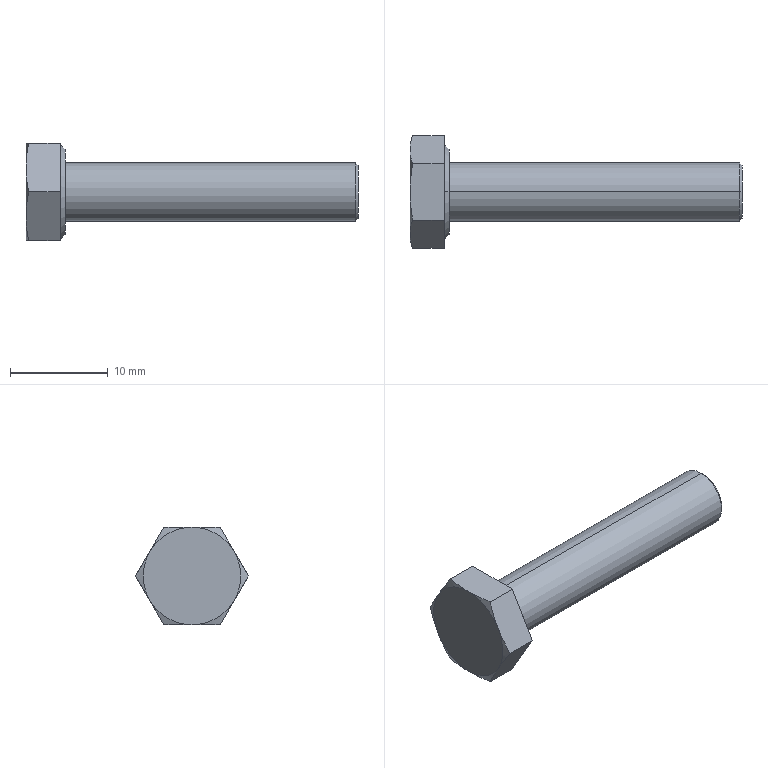Part | SolidWorks | features RevCut 3, Boss 1, Chamfer 1, Extrusion 1, Fillet 1, LPattern 1 | 1 solid | 22 faces | box 34 x 11.547 x 10 mm | volume 1183 mm3 | cone 10 | plane 10 | cylinder 2 | commonest cylinder face diameters 6 x2
STEP:
#1=CARTESIAN_POINT('',(34.,0.,-2.7));
#2=VERTEX_POINT('',#1);
#3=CARTESIAN_POINT('',(34.,0.,2.7));
#4=VERTEX_POINT('',#3);
#5=CARTESIAN_POINT('',(34.,0.,0.));
#6=DIRECTION('',(1.,0.,0.));
#7=DIRECTION('',(0.,0.,-1.));
#8=AXIS2_PLACEMENT_3D('',#5,#6,#7);
#9=CIRCLE('',#8,2.7);
#10=EDGE_CURVE('',#2,#4,#9,.T.);
#11=ORIENTED_EDGE('',*,*,#10,.F.);
#12=CARTESIAN_POINT('',(33.7,0.,-3.));
#13=VERTEX_POINT('',#12);
#14=CARTESIAN_POINT('',(34.,0.,-2.7));
#15=DIRECTION('',(-0.7071,0.,-0.7071));
#16=VECTOR('',#15,1000.);
#17=LINE('',#14,#16);
#18=EDGE_CURVE('',#2,#13,#17,.T.);
#19=ORIENTED_EDGE('',*,*,#18,.T.);
#20=CARTESIAN_POINT('',(33.7,0.,3.));
#21=VERTEX_POINT('',#20);
#22=CARTESIAN_POINT('',(33.7,0.,0.));
#23=DIRECTION('',(-1.,0.,0.));
#24=DIRECTION('',(0.,0.,-1.));
#25=AXIS2_PLACEMENT_3D('',#22,#23,#24);
#26=CIRCLE('',#25,3.);
#27=EDGE_CURVE('',#21,#13,#26,.T.);
#28=ORIENTED_EDGE('',*,*,#27,.F.);
#29=CARTESIAN_POINT('',(34.,0.,2.7));
#30=DIRECTION('',(-0.7071,0.,0.7071));
#31=VECTOR('',#30,1000.);
#32=LINE('',#29,#31);
#33=EDGE_CURVE('',#4,#21,#32,.T.);
#34=ORIENTED_EDGE('',*,*,#33,.F.);
#35=EDGE_LOOP('',(#11,#19,#28,#34));
#36=FACE_OUTER_BOUND('',#35,.T.);
#37=CARTESIAN_POINT('',(34.,0.,0.));
#38=DIRECTION('',(-1.,0.,0.));
#39=DIRECTION('',(0.,0.,1.));
#40=AXIS2_PLACEMENT_3D('',#37,#38,#39);
#41=CONICAL_SURFACE('',#40,2.7,0.7854);
#42=ADVANCED_FACE('',(#36),#41,.T.);
#43=ORIENTED_EDGE('',*,*,#27,.T.);
#44=CARTESIAN_POINT('',(4.,0.,-3.));
#45=VERTEX_POINT('',#44);
#46=CARTESIAN_POINT('',(34.,0.,-3.));
#47=DIRECTION('',(-1.,0.,0.));
#48=VECTOR('',#47,1000.);
#49=LINE('',#46,#48);
#50=EDGE_CURVE('',#13,#45,#49,.T.);
#51=ORIENTED_EDGE('',*,*,#50,.T.);
#52=CARTESIAN_POINT('',(4.,0.,3.));
#53=VERTEX_POINT('',#52);
#54=CARTESIAN_POINT('',(4.,0.,0.));
#55=DIRECTION('',(1.,0.,0.));
#56=DIRECTION('',(0.,0.,-1.));
#57=AXIS2_PLACEMENT_3D('',#54,#55,#56);
#58=CIRCLE('',#57,3.);
#59=EDGE_CURVE('',#45,#53,#58,.T.);
#60=ORIENTED_EDGE('',*,*,#59,.T.);
#61=CARTESIAN_POINT('',(34.,0.,3.));
#62=DIRECTION('',(-1.,0.,0.));
#63=VECTOR('',#62,1000.);
#64=LINE('',#61,#63);
#65=EDGE_CURVE('',#21,#53,#64,.T.);
#66=ORIENTED_EDGE('',*,*,#65,.F.);
#67=EDGE_LOOP('',(#43,#51,#60,#66));
#68=FACE_OUTER_BOUND('',#67,.T.);
#69=CARTESIAN_POINT('',(34.,0.,0.));
#70=DIRECTION('',(-1.,0.,0.));
#71=DIRECTION('',(0.,0.,1.));
#72=AXIS2_PLACEMENT_3D('',#69,#70,#71);
#73=CYLINDRICAL_SURFACE('',#72,3.);
#74=ADVANCED_FACE('',(#68),#73,.T.);
#75=CARTESIAN_POINT('',(4.,0.,4.37));
#76=VERTEX_POINT('',#75);
#77=CARTESIAN_POINT('',(4.,0.,-4.37));
#78=VERTEX_POINT('',#77);
#79=CARTESIAN_POINT('',(4.,0.,0.));
#80=DIRECTION('',(-1.,0.,0.));
#81=DIRECTION('',(0.,0.,1.));
#82=AXIS2_PLACEMENT_3D('',#79,#80,#81);
#83=CIRCLE('',#82,4.37);
#84=EDGE_CURVE('',#76,#78,#83,.T.);
#85=ORIENTED_EDGE('',*,*,#84,.T.);
#86=CARTESIAN_POINT('',(3.5,0.,-4.87));
#87=VERTEX_POINT('',#86);
#88=CARTESIAN_POINT('',(3.5,0.,-4.87));
#89=DIRECTION('',(-0.7071,0.,-0.7071));
#90=VECTOR('',#89,1000.);
#91=LINE('',#88,#90);
#92=EDGE_CURVE('',#78,#87,#91,.T.);
#93=ORIENTED_EDGE('',*,*,#92,.T.);
#94=CARTESIAN_POINT('',(3.5,0.,4.87));
#95=VERTEX_POINT('',#94);
#96=CARTESIAN_POINT('',(3.5,0.,0.));
#97=DIRECTION('',(-1.,0.,0.));
#98=DIRECTION('',(0.,0.,1.));
#99=AXIS2_PLACEMENT_3D('',#96,#97,#98);
#100=CIRCLE('',#99,4.87);
#101=EDGE_CURVE('',#95,#87,#100,.T.);
#102=ORIENTED_EDGE('',*,*,#101,.F.);
#103=CARTESIAN_POINT('',(3.5,0.,4.87));
#104=DIRECTION('',(-0.7071,0.,0.7071));
#105=VECTOR('',#104,1000.);
#106=LINE('',#103,#105);
#107=EDGE_CURVE('',#76,#95,#106,.T.);
#108=ORIENTED_EDGE('',*,*,#107,.F.);
#109=EDGE_LOOP('',(#85,#93,#102,#108));
#110=FACE_OUTER_BOUND('',#109,.T.);
#111=CARTESIAN_POINT('',(3.5,0.,0.));
#112=DIRECTION('',(-1.,0.,0.));
#113=DIRECTION('',(0.,0.,1.));
#114=AXIS2_PLACEMENT_3D('',#111,#112,#113);
#115=CONICAL_SURFACE('',#114,4.87,0.7854);
#116=ADVANCED_FACE('',(#110),#115,.T.);
#117=ORIENTED_EDGE('',*,*,#84,.F.);
#118=CARTESIAN_POINT('',(4.,0.,0.));
#119=DIRECTION('',(-1.,0.,0.));
#120=DIRECTION('',(0.,0.,1.));
#121=AXIS2_PLACEMENT_3D('',#118,#119,#120);
#122=CIRCLE('',#121,4.37);
#123=EDGE_CURVE('',#78,#76,#122,.T.);
#124=ORIENTED_EDGE('',*,*,#123,.F.);
#125=EDGE_LOOP('',(#117,#124));
#126=FACE_OUTER_BOUND('',#125,.T.);
#127=CARTESIAN_POINT('',(4.,0.,0.));
#128=DIRECTION('',(1.,0.,0.));
#129=DIRECTION('',(0.,0.,-1.));
#130=AXIS2_PLACEMENT_3D('',#127,#128,#129);
#131=CIRCLE('',#130,3.);
#132=EDGE_CURVE('',#53,#45,#131,.T.);
#133=ORIENTED_EDGE('',*,*,#132,.F.);
#134=ORIENTED_EDGE('',*,*,#59,.F.);
#135=EDGE_LOOP('',(#133,#134));
#136=FACE_BOUND('',#135,.T.);
#137=CARTESIAN_POINT('',(4.,-8.66,-5.));
#138=DIRECTION('',(1.,0.,0.));
#139=DIRECTION('',(0.,0.,-1.));
#140=AXIS2_PLACEMENT_3D('',#137,#138,#139);
#141=PLANE('',#140);
#142=ADVANCED_FACE('',(#126,#136),#141,.T.);
#143=CARTESIAN_POINT('',(0.2815,-5.774,0.));
#144=VERTEX_POINT('',#143);
#145=CARTESIAN_POINT('',(0.,-4.33,2.5));
#146=VERTEX_POINT('',#145);
#147=CARTESIAN_POINT('',(0.2815,-5.774,0.));
#148=CARTESIAN_POINT('',(0.1064,-5.292,0.8333));
#149=CARTESIAN_POINT('',(0.,-4.811,1.667));
#150=CARTESIAN_POINT('',(0.,-4.33,2.5));
#151=B_SPLINE_CURVE_WITH_KNOTS('',3,(#147,#148,#149,#150),.UNSPECIFIED.,.F.,.F.,(4,4),(0.000000231,0.002887),.UNSPECIFIED.);
#152=EDGE_CURVE('',#144,#146,#151,.T.);
#153=ORIENTED_EDGE('',*,*,#152,.F.);
#154=CARTESIAN_POINT('',(3.5,-5.774,0.));
#155=VERTEX_POINT('',#154);
#156=CARTESIAN_POINT('',(4.,-5.774,0.));
#157=DIRECTION('',(-1.,0.,0.));
#158=VECTOR('',#157,1000.);
#159=LINE('',#156,#158);
#160=EDGE_CURVE('',#155,#144,#159,.T.);
#161=ORIENTED_EDGE('',*,*,#160,.F.);
#162=CARTESIAN_POINT('',(3.5,-2.887,5.));
#163=VERTEX_POINT('',#162);
#164=CARTESIAN_POINT('',(3.5,-2.887,5.));
#165=DIRECTION('',(0.,-0.5,-0.866));
#166=VECTOR('',#165,1000.);
#167=LINE('',#164,#166);
#168=EDGE_CURVE('',#163,#155,#167,.T.);
#169=ORIENTED_EDGE('',*,*,#168,.F.);
#170=CARTESIAN_POINT('',(0.2815,-2.887,5.));
#171=VERTEX_POINT('',#170);
#172=CARTESIAN_POINT('',(4.,-2.887,5.));
#173=DIRECTION('',(-1.,0.,0.));
#174=VECTOR('',#173,1000.);
#175=LINE('',#172,#174);
#176=EDGE_CURVE('',#163,#171,#175,.T.);
#177=ORIENTED_EDGE('',*,*,#176,.T.);
#178=CARTESIAN_POINT('',(0.,-4.33,2.5));
#179=CARTESIAN_POINT('',(0.,-3.849,3.333));
#180=CARTESIAN_POINT('',(0.1064,-3.368,4.167));
#181=CARTESIAN_POINT('',(0.2815,-2.887,5.));
#182=B_SPLINE_CURVE_WITH_KNOTS('',3,(#178,#179,#180,#181),.UNSPECIFIED.,.F.,.F.,(4,4),(0.002887,0.005774),.UNSPECIFIED.);
#183=EDGE_CURVE('',#146,#171,#182,.T.);
#184=ORIENTED_EDGE('',*,*,#183,.F.);
#185=EDGE_LOOP('',(#153,#161,#169,#177,#184));
#186=FACE_OUTER_BOUND('',#185,.T.);
#187=CARTESIAN_POINT('',(4.,-2.887,5.));
#188=DIRECTION('',(0.,0.866,-0.5));
#189=DIRECTION('',(0.,0.5,0.866));
#190=AXIS2_PLACEMENT_3D('',#187,#188,#189);
#191=PLANE('',#190);
#192=ADVANCED_FACE('',(#186),#191,.F.);
#193=CARTESIAN_POINT('',(0.2815,-2.887,-5.));
#194=VERTEX_POINT('',#193);
#195=CARTESIAN_POINT('',(0.,-4.33,-2.5));
#196=VERTEX_POINT('',#195);
#197=CARTESIAN_POINT('',(0.2815,-2.887,-5.));
#198=CARTESIAN_POINT('',(0.1064,-3.368,-4.167));
#199=CARTESIAN_POINT('',(0.,-3.849,-3.333));
#200=CARTESIAN_POINT('',(0.,-4.33,-2.5));
#201=B_SPLINE_CURVE_WITH_KNOTS('',3,(#197,#198,#199,#200),.UNSPECIFIED.,.F.,.F.,(4,4),(0.000000231,0.002887),.UNSPECIFIED.);
#202=EDGE_CURVE('',#194,#196,#201,.T.);
#203=ORIENTED_EDGE('',*,*,#202,.F.);
#204=CARTESIAN_POINT('',(3.5,-2.887,-5.));
#205=VERTEX_POINT('',#204);
#206=CARTESIAN_POINT('',(4.,-2.887,-5.));
#207=DIRECTION('',(-1.,0.,0.));
#208=VECTOR('',#207,1000.);
#209=LINE('',#206,#208);
#210=EDGE_CURVE('',#205,#194,#209,.T.);
#211=ORIENTED_EDGE('',*,*,#210,.F.);
#212=CARTESIAN_POINT('',(3.5,-5.774,0.));
#213=DIRECTION('',(0.,0.5,-0.866));
#214=VECTOR('',#213,1000.);
#215=LINE('',#212,#214);
#216=EDGE_CURVE('',#155,#205,#215,.T.);
#217=ORIENTED_EDGE('',*,*,#216,.F.);
#218=ORIENTED_EDGE('',*,*,#160,.T.);
#219=CARTESIAN_POINT('',(0.,-4.33,-2.5));
#220=CARTESIAN_POINT('',(0.,-4.811,-1.667));
#221=CARTESIAN_POINT('',(0.1064,-5.292,-0.8333));
#222=CARTESIAN_POINT('',(0.2815,-5.774,0.));
#223=B_SPLINE_CURVE_WITH_KNOTS('',3,(#219,#220,#221,#222),.UNSPECIFIED.,.F.,.F.,(4,4),(0.002887,0.005774),.UNSPECIFIED.);
#224=EDGE_CURVE('',#196,#144,#223,.T.);
#225=ORIENTED_EDGE('',*,*,#224,.F.);
#226=EDGE_LOOP('',(#203,#211,#217,#218,#225));
#227=FACE_OUTER_BOUND('',#226,.T.);
#228=CARTESIAN_POINT('',(4.,-5.774,0.));
#229=DIRECTION('',(0.,0.866,0.5));
#230=DIRECTION('',(0.,-0.5,0.866));
#231=AXIS2_PLACEMENT_3D('',#228,#229,#230);
#232=PLANE('',#231);
#233=ADVANCED_FACE('',(#227),#232,.F.);
#234=CARTESIAN_POINT('',(0.2815,2.887,-5.));
#235=VERTEX_POINT('',#234);
#236=CARTESIAN_POINT('',(0.,0.,-5.));
#237=VERTEX_POINT('',#236);
#238=CARTESIAN_POINT('',(0.2815,2.887,-5.));
#239=CARTESIAN_POINT('',(0.1069,1.927,-5.));
#240=CARTESIAN_POINT('',(0.,0.9642,-5.));
#241=CARTESIAN_POINT('',(0.,0.,-5.));
#242=B_SPLINE_CURVE_WITH_KNOTS('',3,(#238,#239,#240,#241),.UNSPECIFIED.,.F.,.F.,(4,4),(0.01041,0.01332),.UNSPECIFIED.);
#243=EDGE_CURVE('',#235,#237,#242,.T.);
#244=ORIENTED_EDGE('',*,*,#243,.F.);
#245=CARTESIAN_POINT('',(3.5,2.887,-5.));
#246=VERTEX_POINT('',#245);
#247=CARTESIAN_POINT('',(4.,2.887,-5.));
#248=DIRECTION('',(-1.,0.,0.));
#249=VECTOR('',#248,1000.);
#250=LINE('',#247,#249);
#251=EDGE_CURVE('',#246,#235,#250,.T.);
#252=ORIENTED_EDGE('',*,*,#251,.F.);
#253=CARTESIAN_POINT('',(3.5,-2.887,-5.));
#254=DIRECTION('',(0.,1.,0.));
#255=VECTOR('',#254,1000.);
#256=LINE('',#253,#255);
#257=EDGE_CURVE('',#205,#246,#256,.T.);
#258=ORIENTED_EDGE('',*,*,#257,.F.);
#259=ORIENTED_EDGE('',*,*,#210,.T.);
#260=CARTESIAN_POINT('',(0.,0.,-5.));
#261=CARTESIAN_POINT('',(0.,-0.4807,-5.));
#262=CARTESIAN_POINT('',(0.02571,-0.962,-5.));
#263=CARTESIAN_POINT('',(0.123,-1.926,-5.));
#264=CARTESIAN_POINT('',(0.1945,-2.409,-5.));
#265=CARTESIAN_POINT('',(0.2815,-2.887,-5.));
#266=B_SPLINE_CURVE_WITH_KNOTS('',3,(#260,#261,#262,#263,#264,#265),.UNSPECIFIED.,.F.,.F.,(4,2,4),(0.01332,0.01477,0.01622),.UNSPECIFIED.);
#267=EDGE_CURVE('',#237,#194,#266,.T.);
#268=ORIENTED_EDGE('',*,*,#267,.F.);
#269=EDGE_LOOP('',(#244,#252,#258,#259,#268));
#270=FACE_OUTER_BOUND('',#269,.T.);
#271=CARTESIAN_POINT('',(4.,-2.887,-5.));
#272=DIRECTION('',(0.,0.,1.));
#273=DIRECTION('',(1.,0.,0.));
#274=AXIS2_PLACEMENT_3D('',#271,#272,#273);
#275=PLANE('',#274);
#276=ADVANCED_FACE('',(#270),#275,.F.);
#277=CARTESIAN_POINT('',(0.2815,5.774,0.));
#278=VERTEX_POINT('',#277);
#279=CARTESIAN_POINT('',(0.,4.33,-2.5));
#280=VERTEX_POINT('',#279);
#281=CARTESIAN_POINT('',(0.2815,5.774,0.));
#282=CARTESIAN_POINT('',(0.1064,5.292,-0.8333));
#283=CARTESIAN_POINT('',(0.,4.811,-1.667));
#284=CARTESIAN_POINT('',(0.,4.33,-2.5));
#285=B_SPLINE_CURVE_WITH_KNOTS('',3,(#281,#282,#283,#284),.UNSPECIFIED.,.F.,.F.,(4,4),(0.000000231,0.002887),.UNSPECIFIED.);
#286=EDGE_CURVE('',#278,#280,#285,.T.);
#287=ORIENTED_EDGE('',*,*,#286,.F.);
#288=CARTESIAN_POINT('',(3.5,5.774,0.));
#289=VERTEX_POINT('',#288);
#290=CARTESIAN_POINT('',(4.,5.774,0.));
#291=DIRECTION('',(-1.,0.,0.));
#292=VECTOR('',#291,1000.);
#293=LINE('',#290,#292);
#294=EDGE_CURVE('',#289,#278,#293,.T.);
#295=ORIENTED_EDGE('',*,*,#294,.F.);
#296=CARTESIAN_POINT('',(3.5,2.887,-5.));
#297=DIRECTION('',(0.,0.5,0.866));
#298=VECTOR('',#297,1000.);
#299=LINE('',#296,#298);
#300=EDGE_CURVE('',#246,#289,#299,.T.);
#301=ORIENTED_EDGE('',*,*,#300,.F.);
#302=ORIENTED_EDGE('',*,*,#251,.T.);
#303=CARTESIAN_POINT('',(0.,4.33,-2.5));
#304=CARTESIAN_POINT('',(0.,3.849,-3.333));
#305=CARTESIAN_POINT('',(0.1064,3.368,-4.167));
#306=CARTESIAN_POINT('',(0.2815,2.887,-5.));
#307=B_SPLINE_CURVE_WITH_KNOTS('',3,(#303,#304,#305,#306),.UNSPECIFIED.,.F.,.F.,(4,4),(0.002887,0.005774),.UNSPECIFIED.);
#308=EDGE_CURVE('',#280,#235,#307,.T.);
#309=ORIENTED_EDGE('',*,*,#308,.F.);
#310=EDGE_LOOP('',(#287,#295,#301,#302,#309));
#311=FACE_OUTER_BOUND('',#310,.T.);
#312=CARTESIAN_POINT('',(4.,2.887,-5.));
#313=DIRECTION('',(0.,-0.866,0.5));
#314=DIRECTION('',(0.,-0.5,-0.866));
#315=AXIS2_PLACEMENT_3D('',#312,#313,#314);
#316=PLANE('',#315);
#317=ADVANCED_FACE('',(#311),#316,.F.);
#318=CARTESIAN_POINT('',(0.2815,2.887,5.));
#319=VERTEX_POINT('',#318);
#320=CARTESIAN_POINT('',(0.,4.33,2.5));
#321=VERTEX_POINT('',#320);
#322=CARTESIAN_POINT('',(0.2815,2.887,5.));
#323=CARTESIAN_POINT('',(0.1064,3.368,4.167));
#324=CARTESIAN_POINT('',(0.,3.849,3.333));
#325=CARTESIAN_POINT('',(0.,4.33,2.5));
#326=B_SPLINE_CURVE_WITH_KNOTS('',3,(#322,#323,#324,#325),.UNSPECIFIED.,.F.,.F.,(4,4),(0.000000231,0.002887),.UNSPECIFIED.);
#327=EDGE_CURVE('',#319,#321,#326,.T.);
#328=ORIENTED_EDGE('',*,*,#327,.F.);
#329=CARTESIAN_POINT('',(3.5,2.887,5.));
#330=VERTEX_POINT('',#329);
#331=CARTESIAN_POINT('',(4.,2.887,5.));
#332=DIRECTION('',(-1.,0.,0.));
#333=VECTOR('',#332,1000.);
#334=LINE('',#331,#333);
#335=EDGE_CURVE('',#330,#319,#334,.T.);
#336=ORIENTED_EDGE('',*,*,#335,.F.);
#337=CARTESIAN_POINT('',(3.5,5.774,0.));
#338=DIRECTION('',(0.,-0.5,0.866));
#339=VECTOR('',#338,1000.);
#340=LINE('',#337,#339);
#341=EDGE_CURVE('',#289,#330,#340,.T.);
#342=ORIENTED_EDGE('',*,*,#341,.F.);
#343=ORIENTED_EDGE('',*,*,#294,.T.);
#344=CARTESIAN_POINT('',(0.,4.33,2.5));
#345=CARTESIAN_POINT('',(0.,4.811,1.667));
#346=CARTESIAN_POINT('',(0.1064,5.292,0.8333));
#347=CARTESIAN_POINT('',(0.2815,5.774,0.));
#348=B_SPLINE_CURVE_WITH_KNOTS('',3,(#344,#345,#346,#347),.UNSPECIFIED.,.F.,.F.,(4,4),(0.002887,0.005774),.UNSPECIFIED.);
#349=EDGE_CURVE('',#321,#278,#348,.T.);
#350=ORIENTED_EDGE('',*,*,#349,.F.);
#351=EDGE_LOOP('',(#328,#336,#342,#343,#350));
#352=FACE_OUTER_BOUND('',#351,.T.);
#353=CARTESIAN_POINT('',(4.,5.774,0.));
#354=DIRECTION('',(0.,-0.866,-0.5));
#355=DIRECTION('',(0.,0.5,-0.866));
#356=AXIS2_PLACEMENT_3D('',#353,#354,#355);
#357=PLANE('',#356);
#358=ADVANCED_FACE('',(#352),#357,.F.);
#359=CARTESIAN_POINT('',(0.,0.,5.));
#360=VERTEX_POINT('',#359);
#361=CARTESIAN_POINT('',(0.2815,-2.887,5.));
#362=CARTESIAN_POINT('',(0.1945,-2.409,5.));
#363=CARTESIAN_POINT('',(0.123,-1.926,5.));
#364=CARTESIAN_POINT('',(0.02571,-0.962,5.));
#365=CARTESIAN_POINT('',(0.,-0.4807,5.));
#366=CARTESIAN_POINT('',(0.,0.,5.));
#367=B_SPLINE_CURVE_WITH_KNOTS('',3,(#361,#362,#363,#364,#365,#366),.UNSPECIFIED.,.F.,.F.,(4,2,4),(0.004911,0.006366,0.00782),.UNSPECIFIED.);
#368=EDGE_CURVE('',#171,#360,#367,.T.);
#369=ORIENTED_EDGE('',*,*,#368,.F.);
#370=ORIENTED_EDGE('',*,*,#176,.F.);
#371=CARTESIAN_POINT('',(3.5,2.887,5.));
#372=DIRECTION('',(0.,-1.,0.));
#373=VECTOR('',#372,1000.);
#374=LINE('',#371,#373);
#375=EDGE_CURVE('',#330,#163,#374,.T.);
#376=ORIENTED_EDGE('',*,*,#375,.F.);
#377=ORIENTED_EDGE('',*,*,#335,.T.);
#378=CARTESIAN_POINT('',(0.,0.,5.));
#379=CARTESIAN_POINT('',(0.,0.9642,5.));
#380=CARTESIAN_POINT('',(0.1069,1.927,5.));
#381=CARTESIAN_POINT('',(0.2815,2.887,5.));
#382=B_SPLINE_CURVE_WITH_KNOTS('',3,(#378,#379,#380,#381),.UNSPECIFIED.,.F.,.F.,(4,4),(0.00782,0.01074),.UNSPECIFIED.);
#383=EDGE_CURVE('',#360,#319,#382,.T.);
#384=ORIENTED_EDGE('',*,*,#383,.F.);
#385=EDGE_LOOP('',(#369,#370,#376,#377,#384));
#386=FACE_OUTER_BOUND('',#385,.T.);
#387=CARTESIAN_POINT('',(4.,2.887,5.));
#388=DIRECTION('',(0.,0.,-1.));
#389=DIRECTION('',(-1.,0.,0.));
#390=AXIS2_PLACEMENT_3D('',#387,#388,#389);
#391=PLANE('',#390);
#392=ADVANCED_FACE('',(#386),#391,.F.);
#393=ORIENTED_EDGE('',*,*,#101,.T.);
#394=CARTESIAN_POINT('',(3.5,0.,0.));
#395=DIRECTION('',(-1.,0.,0.));
#396=DIRECTION('',(0.,0.,1.));
#397=AXIS2_PLACEMENT_3D('',#394,#395,#396);
#398=CIRCLE('',#397,4.87);
#399=EDGE_CURVE('',#87,#95,#398,.T.);
#400=ORIENTED_EDGE('',*,*,#399,.T.);
#401=EDGE_LOOP('',(#393,#400));
#402=FACE_BOUND('',#401,.T.);
#403=ORIENTED_EDGE('',*,*,#168,.T.);
#404=ORIENTED_EDGE('',*,*,#216,.T.);
#405=ORIENTED_EDGE('',*,*,#257,.T.);
#406=ORIENTED_EDGE('',*,*,#300,.T.);
#407=ORIENTED_EDGE('',*,*,#341,.T.);
#408=ORIENTED_EDGE('',*,*,#375,.T.);
#409=EDGE_LOOP('',(#403,#404,#405,#406,#407,#408));
#410=FACE_OUTER_BOUND('',#409,.T.);
#411=CARTESIAN_POINT('',(3.5,4.87,0.));
#412=DIRECTION('',(1.,0.,0.));
#413=DIRECTION('',(0.,0.,-1.));
#414=AXIS2_PLACEMENT_3D('',#411,#412,#413);
#415=PLANE('',#414);
#416=ADVANCED_FACE('',(#402,#410),#415,.T.);
#417=ORIENTED_EDGE('',*,*,#92,.F.);
#418=ORIENTED_EDGE('',*,*,#123,.T.);
#419=ORIENTED_EDGE('',*,*,#107,.T.);
#420=ORIENTED_EDGE('',*,*,#399,.F.);
#421=EDGE_LOOP('',(#417,#418,#419,#420));
#422=FACE_OUTER_BOUND('',#421,.T.);
#423=CARTESIAN_POINT('',(3.5,0.,0.));
#424=DIRECTION('',(-1.,0.,0.));
#425=DIRECTION('',(0.,0.,1.));
#426=AXIS2_PLACEMENT_3D('',#423,#424,#425);
#427=CONICAL_SURFACE('',#426,4.87,0.7854);
#428=ADVANCED_FACE('',(#422),#427,.T.);
#429=ORIENTED_EDGE('',*,*,#267,.T.);
#430=ORIENTED_EDGE('',*,*,#202,.T.);
#431=CARTESIAN_POINT('',(0.,0.,0.));
#432=DIRECTION('',(1.,0.,0.));
#433=DIRECTION('',(0.,0.,-1.));
#434=AXIS2_PLACEMENT_3D('',#431,#432,#433);
#435=CIRCLE('',#434,5.);
#436=EDGE_CURVE('',#196,#237,#435,.T.);
#437=ORIENTED_EDGE('',*,*,#436,.T.);
#438=EDGE_LOOP('',(#429,#430,#437));
#439=FACE_OUTER_BOUND('',#438,.T.);
#440=CARTESIAN_POINT('',(0.,0.,0.));
#441=DIRECTION('',(1.,0.,0.));
#442=DIRECTION('',(0.,0.,-1.));
#443=AXIS2_PLACEMENT_3D('',#440,#441,#442);
#444=CONICAL_SURFACE('',#443,5.,1.222);
#445=ADVANCED_FACE('',(#439),#444,.T.);
#446=ORIENTED_EDGE('',*,*,#224,.T.);
#447=ORIENTED_EDGE('',*,*,#152,.T.);
#448=CARTESIAN_POINT('',(0.,0.,0.));
#449=DIRECTION('',(1.,0.,0.));
#450=DIRECTION('',(0.,0.,-1.));
#451=AXIS2_PLACEMENT_3D('',#448,#449,#450);
#452=CIRCLE('',#451,5.);
#453=EDGE_CURVE('',#146,#196,#452,.T.);
#454=ORIENTED_EDGE('',*,*,#453,.T.);
#455=EDGE_LOOP('',(#446,#447,#454));
#456=FACE_OUTER_BOUND('',#455,.T.);
#457=CARTESIAN_POINT('',(0.,0.,0.));
#458=DIRECTION('',(1.,0.,0.));
#459=DIRECTION('',(0.,0.,-1.));
#460=AXIS2_PLACEMENT_3D('',#457,#458,#459);
#461=CONICAL_SURFACE('',#460,5.,1.222);
#462=ADVANCED_FACE('',(#456),#461,.T.);
#463=ORIENTED_EDGE('',*,*,#183,.T.);
#464=ORIENTED_EDGE('',*,*,#368,.T.);
#465=CARTESIAN_POINT('',(0.,0.,0.));
#466=DIRECTION('',(1.,0.,0.));
#467=DIRECTION('',(0.,0.,-1.));
#468=AXIS2_PLACEMENT_3D('',#465,#466,#467);
#469=CIRCLE('',#468,5.);
#470=EDGE_CURVE('',#360,#146,#469,.T.);
#471=ORIENTED_EDGE('',*,*,#470,.T.);
#472=EDGE_LOOP('',(#463,#464,#471));
#473=FACE_OUTER_BOUND('',#472,.T.);
#474=CARTESIAN_POINT('',(0.,0.,0.));
#475=DIRECTION('',(1.,0.,0.));
#476=DIRECTION('',(0.,0.,-1.));
#477=AXIS2_PLACEMENT_3D('',#474,#475,#476);
#478=CONICAL_SURFACE('',#477,5.,1.222);
#479=ADVANCED_FACE('',(#473),#478,.T.);
#480=ORIENTED_EDGE('',*,*,#327,.T.);
#481=CARTESIAN_POINT('',(0.,0.,0.));
#482=DIRECTION('',(-1.,0.,0.));
#483=DIRECTION('',(0.,0.,1.));
#484=AXIS2_PLACEMENT_3D('',#481,#482,#483);
#485=CIRCLE('',#484,5.);
#486=EDGE_CURVE('',#360,#321,#485,.T.);
#487=ORIENTED_EDGE('',*,*,#486,.F.);
#488=ORIENTED_EDGE('',*,*,#383,.T.);
#489=EDGE_LOOP('',(#480,#487,#488));
#490=FACE_OUTER_BOUND('',#489,.T.);
#491=CARTESIAN_POINT('',(0.,0.,0.));
#492=DIRECTION('',(1.,0.,0.));
#493=DIRECTION('',(0.,0.,-1.));
#494=AXIS2_PLACEMENT_3D('',#491,#492,#493);
#495=CONICAL_SURFACE('',#494,5.,1.222);
#496=ADVANCED_FACE('',(#490),#495,.T.);
#497=ORIENTED_EDGE('',*,*,#286,.T.);
#498=CARTESIAN_POINT('',(0.,0.,0.));
#499=DIRECTION('',(1.,0.,0.));
#500=DIRECTION('',(0.,0.,-1.));
#501=AXIS2_PLACEMENT_3D('',#498,#499,#500);
#502=CIRCLE('',#501,5.);
#503=EDGE_CURVE('',#280,#321,#502,.T.);
#504=ORIENTED_EDGE('',*,*,#503,.T.);
#505=ORIENTED_EDGE('',*,*,#349,.T.);
#506=EDGE_LOOP('',(#497,#504,#505));
#507=FACE_OUTER_BOUND('',#506,.T.);
#508=CARTESIAN_POINT('',(0.,0.,0.));
#509=DIRECTION('',(1.,0.,0.));
#510=DIRECTION('',(0.,0.,-1.));
#511=AXIS2_PLACEMENT_3D('',#508,#509,#510);
#512=CONICAL_SURFACE('',#511,5.,1.222);
#513=ADVANCED_FACE('',(#507),#512,.T.);
#514=ORIENTED_EDGE('',*,*,#243,.T.);
#515=CARTESIAN_POINT('',(0.,0.,0.));
#516=DIRECTION('',(1.,0.,0.));
#517=DIRECTION('',(0.,0.,-1.));
#518=AXIS2_PLACEMENT_3D('',#515,#516,#517);
#519=CIRCLE('',#518,5.);
#520=EDGE_CURVE('',#237,#280,#519,.T.);
#521=ORIENTED_EDGE('',*,*,#520,.T.);
#522=ORIENTED_EDGE('',*,*,#308,.T.);
#523=EDGE_LOOP('',(#514,#521,#522));
#524=FACE_OUTER_BOUND('',#523,.T.);
#525=CARTESIAN_POINT('',(0.,0.,0.));
#526=DIRECTION('',(1.,0.,0.));
#527=DIRECTION('',(0.,0.,-1.));
#528=AXIS2_PLACEMENT_3D('',#525,#526,#527);
#529=CONICAL_SURFACE('',#528,5.,1.222);
#530=ADVANCED_FACE('',(#524),#529,.T.);
#531=ORIENTED_EDGE('',*,*,#520,.F.);
#532=ORIENTED_EDGE('',*,*,#436,.F.);
#533=ORIENTED_EDGE('',*,*,#453,.F.);
#534=ORIENTED_EDGE('',*,*,#470,.F.);
#535=ORIENTED_EDGE('',*,*,#486,.T.);
#536=ORIENTED_EDGE('',*,*,#503,.F.);
#537=EDGE_LOOP('',(#531,#532,#533,#534,#535,#536));
#538=FACE_OUTER_BOUND('',#537,.T.);
#539=CARTESIAN_POINT('',(0.,-8.66,-5.));
#540=DIRECTION('',(1.,0.,0.));
#541=DIRECTION('',(0.,0.,-1.));
#542=AXIS2_PLACEMENT_3D('',#539,#540,#541);
#543=PLANE('',#542);
#544=ADVANCED_FACE('',(#538),#543,.F.);
#545=ORIENTED_EDGE('',*,*,#50,.F.);
#546=CARTESIAN_POINT('',(33.7,0.,0.));
#547=DIRECTION('',(-1.,0.,0.));
#548=DIRECTION('',(0.,0.,-1.));
#549=AXIS2_PLACEMENT_3D('',#546,#547,#548);
#550=CIRCLE('',#549,3.);
#551=EDGE_CURVE('',#13,#21,#550,.T.);
#552=ORIENTED_EDGE('',*,*,#551,.T.);
#553=ORIENTED_EDGE('',*,*,#65,.T.);
#554=ORIENTED_EDGE('',*,*,#132,.T.);
#555=EDGE_LOOP('',(#545,#552,#553,#554));
#556=FACE_OUTER_BOUND('',#555,.T.);
#557=CARTESIAN_POINT('',(34.,0.,0.));
#558=DIRECTION('',(-1.,0.,0.));
#559=DIRECTION('',(0.,0.,1.));
#560=AXIS2_PLACEMENT_3D('',#557,#558,#559);
#561=CYLINDRICAL_SURFACE('',#560,3.);
#562=ADVANCED_FACE('',(#556),#561,.T.);
#563=CARTESIAN_POINT('',(34.,0.,0.));
#564=DIRECTION('',(1.,0.,0.));
#565=DIRECTION('',(0.,0.,-1.));
#566=AXIS2_PLACEMENT_3D('',#563,#564,#565);
#567=CIRCLE('',#566,2.7);
#568=EDGE_CURVE('',#4,#2,#567,.T.);
#569=ORIENTED_EDGE('',*,*,#568,.T.);
#570=ORIENTED_EDGE('',*,*,#10,.T.);
#571=EDGE_LOOP('',(#569,#570));
#572=FACE_OUTER_BOUND('',#571,.T.);
#573=CARTESIAN_POINT('',(34.,0.,0.));
#574=DIRECTION('',(1.,0.,0.));
#575=DIRECTION('',(0.,0.,-1.));
#576=AXIS2_PLACEMENT_3D('',#573,#574,#575);
#577=PLANE('',#576);
#578=ADVANCED_FACE('',(#572),#577,.T.);
#579=ORIENTED_EDGE('',*,*,#18,.F.);
#580=ORIENTED_EDGE('',*,*,#568,.F.);
#581=ORIENTED_EDGE('',*,*,#33,.T.);
#582=ORIENTED_EDGE('',*,*,#551,.F.);
#583=EDGE_LOOP('',(#579,#580,#581,#582));
#584=FACE_OUTER_BOUND('',#583,.T.);
#585=CARTESIAN_POINT('',(34.,0.,0.));
#586=DIRECTION('',(-1.,0.,0.));
#587=DIRECTION('',(0.,0.,1.));
#588=AXIS2_PLACEMENT_3D('',#585,#586,#587);
#589=CONICAL_SURFACE('',#588,2.7,0.7854);
#590=ADVANCED_FACE('',(#584),#589,.T.);
#591=CLOSED_SHELL('',(#42,#74,#116,#142,#192,#233,#276,#317,#358,#392,#416,#428,#445,#462,#479,#496,#513,#530,#544,#562,#578,#590));
#592=MANIFOLD_SOLID_BREP('',#591);
#593=CARTESIAN_POINT('',(0.,0.,0.));
#594=DIRECTION('',(0.,0.,1.));
#595=DIRECTION('',(1.,0.,0.));
#596=AXIS2_PLACEMENT_3D('',#593,#594,#595);
#597=(LENGTH_UNIT()NAMED_UNIT(*)SI_UNIT(.MILLI.,.METRE.));
#598=UNCERTAINTY_MEASURE_WITH_UNIT(LENGTH_MEASURE(0.00001),#597,'','');
#599=(NAMED_UNIT(*)PLANE_ANGLE_UNIT()SI_UNIT($,.RADIAN.));
#600=(NAMED_UNIT(*)SI_UNIT($,.STERADIAN.)SOLID_ANGLE_UNIT());
#601=(GEOMETRIC_REPRESENTATION_CONTEXT(3)GLOBAL_UNCERTAINTY_ASSIGNED_CONTEXT((#598))GLOBAL_UNIT_ASSIGNED_CONTEXT((#597,#599,#600))REPRESENTATION_CONTEXT('',''));
#602=ADVANCED_BREP_SHAPE_REPRESENTATION('',(#592,#596),#601);